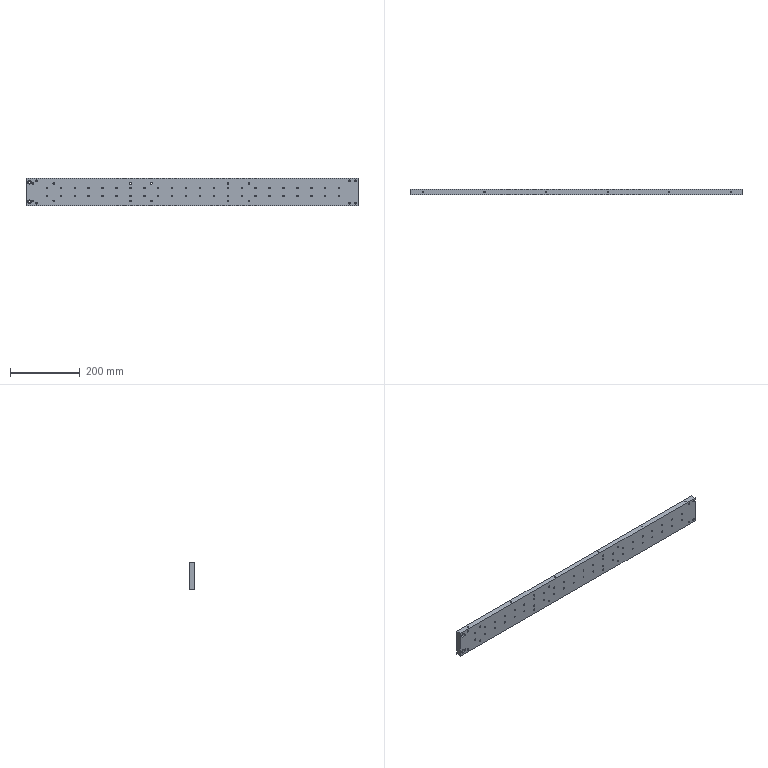Part | STEP file | 866-BDO024-95-01A_default | 1 solid | 197 faces | box 954 x 15 x 80 mm | volume 1055067 mm3 | cylinder 160 | cone 24 | plane 13 | commonest cylinder face diameters 4 x92 5 x36 3.3 x24 6.6 x4 11 x4